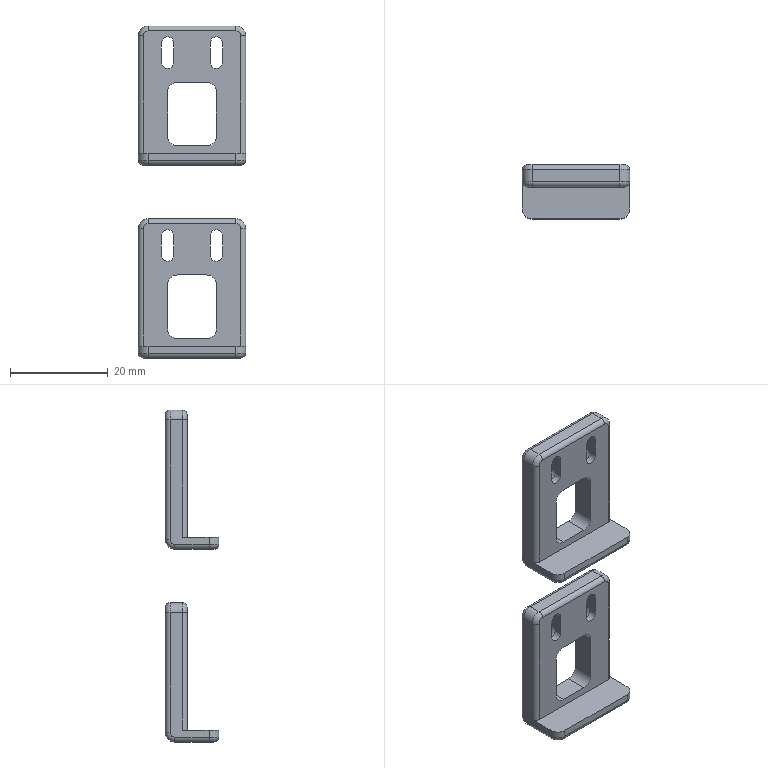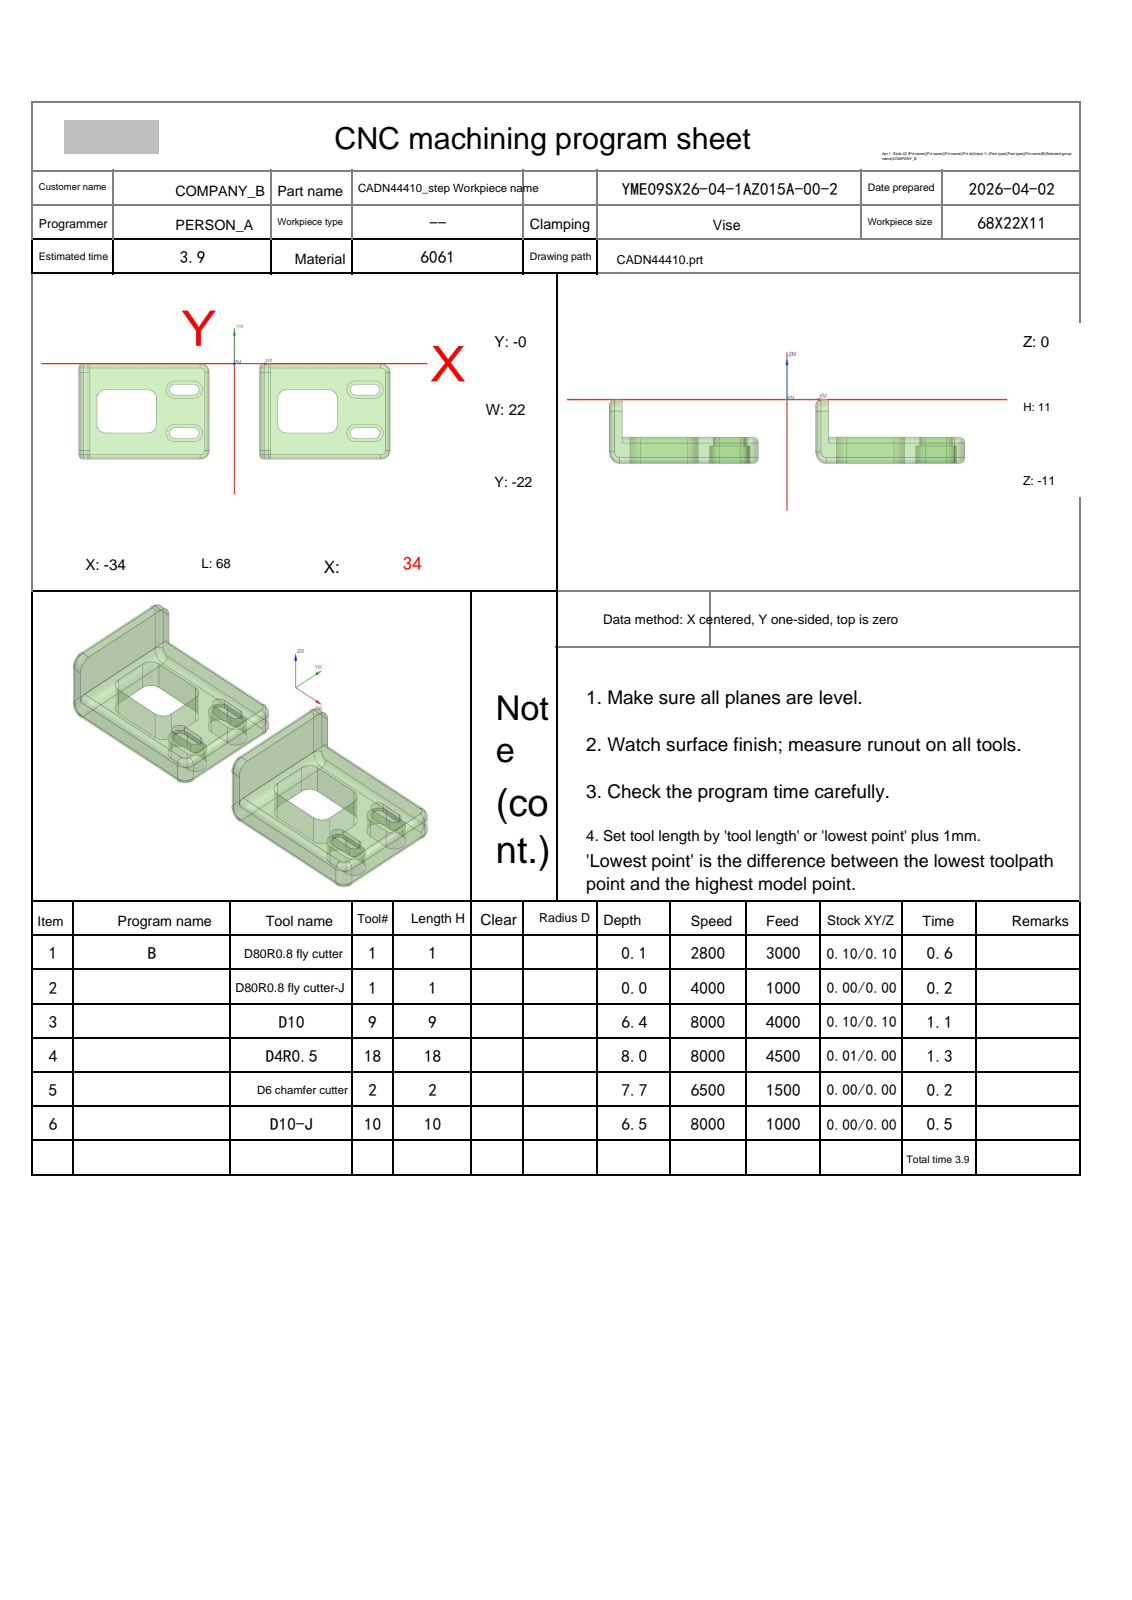NC program | NX | posted by the shop | part box 22 x 11 x 68 mm
Lines 1 to 1003 of 3177:
%
O0001
(Machine time: 5.00 MIN)
(===Total Tool:5===)
(T1=D80R0.8 fly cutter D=80.  R=0.8 H01 Z=0.    )
(T9=D10     D=10.  R=0.   D-  H09 Z=-6.4  )
(T18=D4R0.5 D=4.   R=0.5  D-  H18 Z=-8.   )
(T2=D6 chamfer cutter   D=6.   R=0.   D-  H02 Z=-7.7  )
(T10=D10-J  D=10.  R=0.   D10 H10 Z=-6.5  )
G80 G90 G17 G49 G40
G91 G28 Z0
M01
N1 T01 M06
(D80R0.8 fly cutter D=80. R=0.8 H=01 ce=0.10 di=0.10)
G00 G90 G54 X-86.097 Y-11. M03 S2800
G43 H01 Z20.
M08
Z5.513
G01 Z3.513 F3000.
X-74.097
X74.097
X86.097
Z5.513
G00 X-86.097
Z5.025
G01 Z3.025
X-74.097
X74.097
X86.097
Z5.025
G00 X-86.097
Z4.538
G01 Z2.538
X-74.097
X74.097
X86.097
Z4.538
G00 X-86.097
Z4.05
G01 Z2.05
X-74.097
X74.097
X86.097
Z4.05
G00 Z20.
X-86.097
Z3.563
G01 Z1.563
X-74.097
X74.097
X86.097
Z3.563
G00 Z20.
X-86.097
Z3.075
G01 Z1.075
X-74.097
X74.097
X86.097
Z3.075
G00 Z20.
X-86.097
Z2.588
G01 Z.588
X-74.097
X74.097
X86.097
Z2.588
G00 Z20.
X-86.097
Z2.1
G01 Z.1
X-74.097
X74.097
X86.097
Z2.1
G00 Z20.
G91 G28 Z0.0
M05
M09
G91 G28 Z0.0
M01
N2 T01 M06
(D80R0.8 fly cutter-J D=80. R=0.8 H=01 ce=0.00 di=0.00)
G00 G90 G54 X-85.999 Y-11. M03 S4000
G43 H01 Z20.
M08
Z2.
G01 Z0.0 F1000.
X-73.999
X73.999
X85.999
Z2.
G00 Z20.
G91 G28 Z0.0
M05
M09
G91 G28 Z0.0
M01
N3 T09 M06
(D10  D=10. R=0. H=09 ce=0.10 di=0.10)
G00 G90 G54 X-13.025 Y7. M03 S8000
G43 H09 Z13.5
M08
Z.918
G01 Z-.582 F4000.
Y3.9
X-7.5
G02 X-7.1 Y3.886 I0.0 J-5.9
X-5.689 Y3.615 I-.4 J-5.886
G01 X2.725 Y3.792
G03 X.4 Y-1. I3.775 J-4.792
G01 Y-21.
G03 X2.725 Y-25.792 I6.1 J0.0
G01 X-5.689 Y-25.615
X-5.705 Y-25.62
G02 X-7.5 Y-25.9 I-1.795 J5.62
G01 X-26.45
Y3.9
X-16.06
G02 X-15.228 Y3.455 I0.0 J-1.
G01 X-10.822 Y-3.155
G03 X-9.99 Y-3.6 I.832 J.555
G01 X-8.098
G02 X-7.1 Y-4.598 I-.002 J-1.
G01 Y-17.402
G02 X-8.098 Y-18.4 I-1. J.002
G01 X-17.952
G02 X-18.95 Y-17.402 I.002 J1.
G01 Y-4.598
G02 X-17.952 Y-3.6 I1. J-.002
G01 X-15.844
G02 X-14.984 Y-4.089 I0.0 J-1.
G01 X-12.827 Y-7.714
G03 X-12.284 Y-8.151 I.859 J.512
G02 X-11.6 Y-9.098 I-.316 J-.949
G01 Y-12.902
G02 X-12.598 Y-13.9 I-1. J.002
G01 X-13.452
G02 X-14.45 Y-12.902 I.002 J1.
G01 Y-9.098
G02 X-13.452 Y-8.1 I1. J-.002
G01 X-13.025
X-12.598
X-12.525 Y-8.103
X-12.3 Y-5.111
Z.918
G00 X-13.025 Y7.
Z.336
G01 Z-1.164
Y3.9
X-7.5
G02 X-7.1 Y3.886 I0.0 J-5.9
X-5.689 Y3.615 I-.4 J-5.886
G01 X2.725 Y3.792
G03 X.4 Y-1. I3.775 J-4.792
G01 Y-21.
G03 X2.725 Y-25.792 I6.1 J0.0
G01 X-5.689 Y-25.615
X-5.705 Y-25.62
G02 X-7.5 Y-25.9 I-1.795 J5.62
G01 X-26.45
Y3.9
X-16.06
G02 X-15.228 Y3.455 I0.0 J-1.
G01 X-10.822 Y-3.155
G03 X-9.99 Y-3.6 I.832 J.555
G01 X-8.098
G02 X-7.1 Y-4.598 I-.002 J-1.
G01 Y-17.402
G02 X-8.098 Y-18.4 I-1. J.002
G01 X-17.952
G02 X-18.95 Y-17.402 I.002 J1.
G01 Y-4.598
G02 X-17.952 Y-3.6 I1. J-.002
G01 X-15.844
G02 X-14.984 Y-4.089 I0.0 J-1.
G01 X-12.827 Y-7.714
G03 X-12.284 Y-8.151 I.859 J.512
G02 X-11.6 Y-9.098 I-.316 J-.949
G01 Y-12.902
G02 X-12.598 Y-13.9 I-1. J.002
G01 X-13.452
G02 X-14.45 Y-12.902 I.002 J1.
G01 Y-9.098
G02 X-13.452 Y-8.1 I1. J-.002
G01 X-13.025
X-12.598
X-12.525 Y-8.103
X-12.3 Y-5.111
Z.336
G00 X-13.025 Y7.
Z-.245
G01 Z-1.745
Y3.9
X-7.5
G02 X-7.1 Y3.886 I0.0 J-5.9
X-5.689 Y3.615 I-.4 J-5.886
G01 X2.725 Y3.792
G03 X.4 Y-1. I3.775 J-4.792
G01 Y-21.
G03 X2.725 Y-25.792 I6.1 J0.0
G01 X-5.689 Y-25.615
X-5.705 Y-25.62
G02 X-7.5 Y-25.9 I-1.795 J5.62
G01 X-26.45
Y3.9
X-16.06
G02 X-15.228 Y3.455 I0.0 J-1.
G01 X-10.822 Y-3.155
G03 X-9.99 Y-3.6 I.832 J.555
G01 X-8.098
G02 X-7.1 Y-4.598 I-.002 J-1.
G01 Y-17.402
G02 X-8.098 Y-18.4 I-1. J.002
G01 X-17.952
G02 X-18.95 Y-17.402 I.002 J1.
G01 Y-4.598
G02 X-17.952 Y-3.6 I1. J-.002
G01 X-15.844
G02 X-14.984 Y-4.089 I0.0 J-1.
G01 X-12.827 Y-7.714
G03 X-12.284 Y-8.151 I.859 J.512
G02 X-11.6 Y-9.098 I-.316 J-.949
G01 Y-12.902
G02 X-12.598 Y-13.9 I-1. J.002
G01 X-13.452
G02 X-14.45 Y-12.902 I.002 J1.
G01 Y-9.098
G02 X-13.452 Y-8.1 I1. J-.002
G01 X-13.025
X-12.598
X-12.525 Y-8.103
X-12.3 Y-5.111
Z-.245
G00 X-13.025 Y7.
Z-.827
G01 Z-2.327
Y3.9
X-7.5
G02 X-7.1 Y3.886 I0.0 J-5.9
X-5.689 Y3.615 I-.4 J-5.886
G01 X2.725 Y3.792
G03 X.4 Y-1. I3.775 J-4.792
G01 Y-21.
G03 X2.725 Y-25.792 I6.1 J0.0
G01 X-5.689 Y-25.615
X-5.705 Y-25.62
G02 X-7.5 Y-25.9 I-1.795 J5.62
G01 X-26.45
Y3.9
X-16.06
G02 X-15.228 Y3.455 I0.0 J-1.
G01 X-10.822 Y-3.155
G03 X-9.99 Y-3.6 I.832 J.555
G01 X-8.098
G02 X-7.1 Y-4.598 I-.002 J-1.
G01 Y-17.402
G02 X-8.098 Y-18.4 I-1. J.002
G01 X-17.952
G02 X-18.95 Y-17.402 I.002 J1.
G01 Y-4.598
G02 X-17.952 Y-3.6 I1. J-.002
G01 X-15.844
G02 X-14.984 Y-4.089 I0.0 J-1.
G01 X-12.827 Y-7.714
G03 X-12.284 Y-8.151 I.859 J.512
G02 X-11.6 Y-9.098 I-.316 J-.949
G01 Y-12.902
G02 X-12.598 Y-13.9 I-1. J.002
G01 X-13.452
G02 X-14.45 Y-12.902 I.002 J1.
G01 Y-9.098
G02 X-13.452 Y-8.1 I1. J-.002
G01 X-13.025
X-12.598
X-12.525 Y-8.103
X-12.3 Y-5.111
Z-.827
G00 X-13.025 Y7.
Z-1.409
G01 Z-2.909
Y3.9
X-7.5
G02 X-7.1 Y3.886 I0.0 J-5.9
X-5.689 Y3.615 I-.4 J-5.886
G01 X2.725 Y3.792
G03 X.4 Y-1. I3.775 J-4.792
G01 Y-21.
G03 X2.725 Y-25.792 I6.1 J0.0
G01 X-5.689 Y-25.615
X-5.705 Y-25.62
G02 X-7.5 Y-25.9 I-1.795 J5.62
G01 X-26.45
Y3.9
X-16.06
G02 X-15.228 Y3.455 I0.0 J-1.
G01 X-10.822 Y-3.155
G03 X-9.99 Y-3.6 I.832 J.555
G01 X-8.098
G02 X-7.1 Y-4.598 I-.002 J-1.
G01 Y-17.402
G02 X-8.098 Y-18.4 I-1. J.002
G01 X-17.952
G02 X-18.95 Y-17.402 I.002 J1.
G01 Y-4.598
G02 X-17.952 Y-3.6 I1. J-.002
G01 X-15.844
G02 X-14.984 Y-4.089 I0.0 J-1.
G01 X-12.827 Y-7.714
G03 X-12.284 Y-8.151 I.859 J.512
G02 X-11.6 Y-9.098 I-.316 J-.949
G01 Y-12.902
G02 X-12.598 Y-13.9 I-1. J.002
G01 X-13.452
G02 X-14.45 Y-12.902 I.002 J1.
G01 Y-9.098
G02 X-13.452 Y-8.1 I1. J-.002
G01 X-13.025
X-12.598
X-12.525 Y-8.103
X-12.3 Y-5.111
Z-1.409
G00 X-13.025 Y7.
Z-1.991
G01 Z-3.491
Y3.9
X-7.5
G02 X-7.1 Y3.886 I0.0 J-5.9
X-5.689 Y3.615 I-.4 J-5.886
G01 X2.725 Y3.792
G03 X.4 Y-1. I3.775 J-4.792
G01 Y-21.
G03 X2.725 Y-25.792 I6.1 J0.0
G01 X-5.689 Y-25.615
X-5.705 Y-25.62
G02 X-7.5 Y-25.9 I-1.795 J5.62
G01 X-26.45
Y3.9
X-16.06
G02 X-15.228 Y3.455 I0.0 J-1.
G01 X-10.822 Y-3.155
G03 X-9.99 Y-3.6 I.832 J.555
G01 X-8.098
G02 X-7.1 Y-4.598 I-.002 J-1.
G01 Y-17.402
G02 X-8.098 Y-18.4 I-1. J.002
G01 X-17.952
G02 X-18.95 Y-17.402 I.002 J1.
G01 Y-4.598
G02 X-17.952 Y-3.6 I1. J-.002
G01 X-15.844
G02 X-14.984 Y-4.089 I0.0 J-1.
G01 X-12.827 Y-7.714
G03 X-12.284 Y-8.151 I.859 J.512
G02 X-11.6 Y-9.098 I-.316 J-.949
G01 Y-12.902
G02 X-12.598 Y-13.9 I-1. J.002
G01 X-13.452
G02 X-14.45 Y-12.902 I.002 J1.
G01 Y-9.098
G02 X-13.452 Y-8.1 I1. J-.002
G01 X-13.025
X-12.598
X-12.525 Y-8.103
X-12.3 Y-5.111
Z-1.991
G00 X-13.025 Y7.
Z-2.573
G01 Z-4.073
Y3.9
X-7.5
G02 X-7.1 Y3.886 I0.0 J-5.9
X-5.689 Y3.615 I-.4 J-5.886
G01 X2.725 Y3.792
G03 X.4 Y-1. I3.775 J-4.792
G01 Y-21.
G03 X2.725 Y-25.792 I6.1 J0.0
G01 X-5.689 Y-25.615
X-5.705 Y-25.62
G02 X-7.5 Y-25.9 I-1.795 J5.62
G01 X-26.45
Y3.9
X-16.06
G02 X-15.228 Y3.455 I0.0 J-1.
G01 X-10.822 Y-3.155
G03 X-9.99 Y-3.6 I.832 J.555
G01 X-8.098
G02 X-7.1 Y-4.598 I-.002 J-1.
G01 Y-17.402
G02 X-8.098 Y-18.4 I-1. J.002
G01 X-17.952
G02 X-18.95 Y-17.402 I.002 J1.
G01 Y-4.598
G02 X-17.952 Y-3.6 I1. J-.002
G01 X-15.844
G02 X-14.984 Y-4.089 I0.0 J-1.
G01 X-12.827 Y-7.714
G03 X-12.284 Y-8.151 I.859 J.512
G02 X-11.6 Y-9.098 I-.316 J-.949
G01 Y-12.902
G02 X-12.598 Y-13.9 I-1. J.002
G01 X-13.452
G02 X-14.45 Y-12.902 I.002 J1.
G01 Y-9.098
G02 X-13.452 Y-8.1 I1. J-.002
G01 X-13.025
X-12.598
X-12.525 Y-8.103
X-12.3 Y-5.111
Z-2.573
G00 X-13.025 Y7.
Z-3.155
G01 Z-4.655
Y3.9
X-7.5
G02 X-7.1 Y3.886 I0.0 J-5.9
X-5.689 Y3.615 I-.4 J-5.886
G01 X2.725 Y3.792
G03 X.4 Y-1. I3.775 J-4.792
G01 Y-21.
G03 X2.725 Y-25.792 I6.1 J0.0
G01 X-5.689 Y-25.615
X-5.705 Y-25.62
G02 X-7.5 Y-25.9 I-1.795 J5.62
G01 X-26.45
Y3.9
X-16.06
G02 X-15.228 Y3.455 I0.0 J-1.
G01 X-10.822 Y-3.155
G03 X-9.99 Y-3.6 I.832 J.555
G01 X-8.098
G02 X-7.1 Y-4.598 I-.002 J-1.
G01 Y-17.402
G02 X-8.098 Y-18.4 I-1. J.002
G01 X-17.952
G02 X-18.95 Y-17.402 I.002 J1.
G01 Y-4.598
G02 X-17.952 Y-3.6 I1. J-.002
G01 X-15.844
G02 X-14.984 Y-4.089 I0.0 J-1.
G01 X-12.827 Y-7.714
G03 X-12.284 Y-8.151 I.859 J.512
G02 X-11.6 Y-9.098 I-.316 J-.949
G01 Y-12.902
G02 X-12.598 Y-13.9 I-1. J.002
G01 X-13.452
G02 X-14.45 Y-12.902 I.002 J1.
G01 Y-9.098
G02 X-13.452 Y-8.1 I1. J-.002
G01 X-13.025
X-12.598
X-12.525 Y-8.103
X-12.3 Y-5.111
Z-3.155
G00 X-13.025 Y7.
Z-3.736
G01 Z-5.236
Y3.9
X-7.5
G02 X-7.1 Y3.886 I0.0 J-5.9
X-5.689 Y3.615 I-.4 J-5.886
G01 X2.725 Y3.792
G03 X.4 Y-1. I3.775 J-4.792
G01 Y-21.
G03 X2.725 Y-25.792 I6.1 J0.0
G01 X-5.689 Y-25.615
X-5.705 Y-25.62
G02 X-7.5 Y-25.9 I-1.795 J5.62
G01 X-26.45
Y3.9
X-16.06
G02 X-15.228 Y3.455 I0.0 J-1.
G01 X-10.822 Y-3.155
G03 X-9.99 Y-3.6 I.832 J.555
G01 X-8.098
G02 X-7.1 Y-4.598 I-.002 J-1.
G01 Y-17.402
G02 X-8.098 Y-18.4 I-1. J.002
G01 X-17.952
G02 X-18.95 Y-17.402 I.002 J1.
G01 Y-4.598
G02 X-17.952 Y-3.6 I1. J-.002
G01 X-15.844
G02 X-14.984 Y-4.089 I0.0 J-1.
G01 X-12.827 Y-7.714
G03 X-12.284 Y-8.151 I.859 J.512
G02 X-11.6 Y-9.098 I-.316 J-.949
G01 Y-12.902
G02 X-12.598 Y-13.9 I-1. J.002
G01 X-13.452
G02 X-14.45 Y-12.902 I.002 J1.
G01 Y-9.098
G02 X-13.452 Y-8.1 I1. J-.002
G01 X-13.025
X-12.598
X-12.525 Y-8.103
X-12.3 Y-5.111
Z-3.736
G00 X-13.025 Y7.
Z-4.318
G01 Z-5.818
Y3.9
X-7.5
G02 X-7.1 Y3.886 I0.0 J-5.9
X-5.689 Y3.615 I-.4 J-5.886
G01 X2.725 Y3.792
G03 X.4 Y-1. I3.775 J-4.792
G01 Y-21.
G03 X2.725 Y-25.792 I6.1 J0.0
G01 X-5.689 Y-25.615
X-5.705 Y-25.62
G02 X-7.5 Y-25.9 I-1.795 J5.62
G01 X-26.45
Y3.9
X-16.06
G02 X-15.228 Y3.455 I0.0 J-1.
G01 X-10.822 Y-3.155
G03 X-9.99 Y-3.6 I.832 J.555
G01 X-8.098
G02 X-7.1 Y-4.598 I-.002 J-1.
G01 Y-17.402
G02 X-8.098 Y-18.4 I-1. J.002
G01 X-17.952
G02 X-18.95 Y-17.402 I.002 J1.
G01 Y-4.598
G02 X-17.952 Y-3.6 I1. J-.002
G01 X-15.844
G02 X-14.984 Y-4.089 I0.0 J-1.
G01 X-12.827 Y-7.714
G03 X-12.284 Y-8.151 I.859 J.512
G02 X-11.6 Y-9.098 I-.316 J-.949
G01 Y-12.902
G02 X-12.598 Y-13.9 I-1. J.002
G01 X-13.452
G02 X-14.45 Y-12.902 I.002 J1.
G01 Y-9.098
G02 X-13.452 Y-8.1 I1. J-.002
G01 X-13.025
X-12.598
X-12.525 Y-8.103
X-12.3 Y-5.111
Z-4.318
G00 X-13.025 Y7.
Z-4.9
G01 Z-6.4
Y3.9
X-7.5
G02 X-7.1 Y3.886 I0.0 J-5.9
X-5.689 Y3.615 I-.4 J-5.886
G01 X2.725 Y3.792
G03 X.4 Y-1. I3.775 J-4.792
G01 Y-21.
G03 X2.725 Y-25.792 I6.1 J0.0
G01 X-5.689 Y-25.615
X-5.705 Y-25.62
G02 X-7.5 Y-25.9 I-1.795 J5.62
G01 X-26.45
Y3.9
X-16.06
G02 X-15.228 Y3.455 I0.0 J-1.
G01 X-10.822 Y-3.155
G03 X-9.99 Y-3.6 I.832 J.555
G01 X-8.098
G02 X-7.1 Y-4.598 I-.002 J-1.
G01 Y-17.402
G02 X-8.098 Y-18.4 I-1. J.002
G01 X-17.952
G02 X-18.95 Y-17.402 I.002 J1.
G01 Y-4.598
G02 X-17.952 Y-3.6 I1. J-.002
G01 X-15.844
G02 X-14.984 Y-4.089 I0.0 J-1.
G01 X-12.827 Y-7.714
G03 X-12.284 Y-8.151 I.859 J.512
G02 X-11.6 Y-9.098 I-.316 J-.949
G01 Y-12.902
G02 X-12.598 Y-13.9 I-1. J.002
G01 X-13.452
G02 X-14.45 Y-12.902 I.002 J1.
G01 Y-9.098
G02 X-13.452 Y-8.1 I1. J-.002
G01 X-13.025
X-12.598
X-12.525 Y-8.103
X-12.3 Y-5.111
Z-4.9
G00 Z13.5
X41. Y-11.
Z.918
G01 Z-.582
X37.9
Y-20.
G02 X32. Y-25.9 I-5.9 J0.0
G01 X13.05
Y3.9
X32.
G02 X37.9 Y-2. I0.0 J-5.9
G01 Y-7.965
G02 X37.455 Y-8.797 I-1. J0.0
G01 X30.845 Y-13.203
G03 X30.4 Y-14.035 I.555 J-.832
G01 Y-17.402
G02 X29.402 Y-18.4 I-1. J.002
G01 X21.548
G02 X20.55 Y-17.402 I.002 J1.
G01 Y-4.598
G02 X21.548 Y-3.6 I1. J-.002
G01 X29.402
G02 X30.4 Y-4.598 I-.002 J-1.
G01 Y-8.336
G02 X30.107 Y-9.043 I-1. J0.0
G01 X26.182 Y-12.968
G03 X25.897 Y-13.55 I.707 J-.707
G02 X25.502 Y-13.9 I-.397 J.05
G01 X25.448
G02 X25.05 Y-13.502 I.002 J.4
G01 Y-8.498
G02 X25.448 Y-8.1 I.4 J-.002
G01 X25.502
G02 X25.9 Y-8.498 I-.002 J-.4
G01 Y-11.
Y-11.5
X28.9
Z.918
G00 X41. Y-11.
Z.336
G01 Z-1.164
X37.9
Y-20.
G02 X32. Y-25.9 I-5.9 J0.0
G01 X13.05
Y3.9
X32.
G02 X37.9 Y-2. I0.0 J-5.9
G01 Y-7.965
G02 X37.455 Y-8.797 I-1. J0.0
G01 X30.845 Y-13.203
G03 X30.4 Y-14.035 I.555 J-.832
G01 Y-17.402
G02 X29.402 Y-18.4 I-1. J.002
G01 X21.548
G02 X20.55 Y-17.402 I.002 J1.
G01 Y-4.598
G02 X21.548 Y-3.6 I1. J-.002
G01 X29.402
G02 X30.4 Y-4.598 I-.002 J-1.
G01 Y-8.336
G02 X30.107 Y-9.043 I-1. J0.0
G01 X26.182 Y-12.968
G03 X25.897 Y-13.55 I.707 J-.707
G02 X25.502 Y-13.9 I-.397 J.05
G01 X25.448
G02 X25.05 Y-13.502 I.002 J.4
G01 Y-8.498
G02 X25.448 Y-8.1 I.4 J-.002
G01 X25.502
G02 X25.9 Y-8.498 I-.002 J-.4
G01 Y-11.
Y-11.5
X28.9
Z.336
G00 X41. Y-11.
Z-.245
G01 Z-1.745
X37.9
Y-20.
G02 X32. Y-25.9 I-5.9 J0.0
G01 X13.05
Y3.9
X32.
G02 X37.9 Y-2. I0.0 J-5.9
G01 Y-7.965
G02 X37.455 Y-8.797 I-1. J0.0
G01 X30.845 Y-13.203
G03 X30.4 Y-14.035 I.555 J-.832
G01 Y-17.402
G02 X29.402 Y-18.4 I-1. J.002
G01 X21.548
G02 X20.55 Y-17.402 I.002 J1.
G01 Y-4.598
G02 X21.548 Y-3.6 I1. J-.002
G01 X29.402
G02 X30.4 Y-4.598 I-.002 J-1.
G01 Y-8.336
G02 X30.107 Y-9.043 I-1. J0.0
G01 X26.182 Y-12.968
G03 X25.897 Y-13.55 I.707 J-.707
G02 X25.502 Y-13.9 I-.397 J.05
G01 X25.448
G02 X25.05 Y-13.502 I.002 J.4
G01 Y-8.498
G02 X25.448 Y-8.1 I.4 J-.002
G01 X25.502
G02 X25.9 Y-8.498 I-.002 J-.4
G01 Y-11.
Y-11.5
X28.9
Z-.245
G00 X41. Y-11.
Z-.827
G01 Z-2.327
X37.9
Y-20.
G02 X32. Y-25.9 I-5.9 J0.0
G01 X13.05
Y3.9
X32.
G02 X37.9 Y-2. I0.0 J-5.9
G01 Y-7.965
G02 X37.455 Y-8.797 I-1. J0.0
G01 X30.845 Y-13.203
G03 X30.4 Y-14.035 I.555 J-.832
G01 Y-17.402
G02 X29.402 Y-18.4 I-1. J.002
G01 X21.548
G02 X20.55 Y-17.402 I.002 J1.
G01 Y-4.598
G02 X21.548 Y-3.6 I1. J-.002
G01 X29.402
G02 X30.4 Y-4.598 I-.002 J-1.
G01 Y-8.336
G02 X30.107 Y-9.043 I-1. J0.0
G01 X26.182 Y-12.968
G03 X25.897 Y-13.55 I.707 J-.707
G02 X25.502 Y-13.9 I-.397 J.05
G01 X25.448
G02 X25.05 Y-13.502 I.002 J.4
G01 Y-8.498
G02 X25.448 Y-8.1 I.4 J-.002
G01 X25.502
G02 X25.9 Y-8.498 I-.002 J-.4
G01 Y-11.
Y-11.5
X28.9
Z-.827
G00 X41. Y-11.
Z-1.409
G01 Z-2.909
X37.9
Y-20.
G02 X32. Y-25.9 I-5.9 J0.0
G01 X13.05
Y3.9
X32.
G02 X37.9 Y-2. I0.0 J-5.9
G01 Y-7.965
G02 X37.455 Y-8.797 I-1. J0.0
G01 X30.845 Y-13.203
G03 X30.4 Y-14.035 I.555 J-.832
G01 Y-17.402
G02 X29.402 Y-18.4 I-1. J.002
G01 X21.548
G02 X20.55 Y-17.402 I.002 J1.
G01 Y-4.598
G02 X21.548 Y-3.6 I1. J-.002
G01 X29.402
G02 X30.4 Y-4.598 I-.002 J-1.
G01 Y-8.336
G02 X30.107 Y-9.043 I-1. J0.0
G01 X26.182 Y-12.968
G03 X25.897 Y-13.55 I.707 J-.707
G02 X25.502 Y-13.9 I-.397 J.05
G01 X25.448
G02 X25.05 Y-13.502 I.002 J.4
G01 Y-8.498
G02 X25.448 Y-8.1 I.4 J-.002
G01 X25.502
G02 X25.9 Y-8.498 I-.002 J-.4
G01 Y-11.
Y-11.5
X28.9
Z-1.409
G00 X41. Y-11.
Z-1.991
G01 Z-3.491
X37.9
Y-20.
G02 X32. Y-25.9 I-5.9 J0.0
G01 X13.05
Y3.9
X32.
G02 X37.9 Y-2. I0.0 J-5.9
G01 Y-7.965
G02 X37.455 Y-8.797 I-1. J0.0
G01 X30.845 Y-13.203
G03 X30.4 Y-14.035 I.555 J-.832
G01 Y-17.402
G02 X29.402 Y-18.4 I-1. J.002
G01 X21.548
G02 X20.55 Y-17.402 I.002 J1.
G01 Y-4.598
G02 X21.548 Y-3.6 I1. J-.002
G01 X29.402
G02 X30.4 Y-4.598 I-.002 J-1.
G01 Y-8.336
G02 X30.107 Y-9.043 I-1. J0.0
G01 X26.182 Y-12.968
G03 X25.897 Y-13.55 I.707 J-.707
G02 X25.502 Y-13.9 I-.397 J.05
G01 X25.448
G02 X25.05 Y-13.502 I.002 J.4
G01 Y-8.498
G02 X25.448 Y-8.1 I.4 J-.002
G01 X25.502
G02 X25.9 Y-8.498 I-.002 J-.4
G01 Y-11.
Y-11.5
X28.9
Z-1.991
G00 X41. Y-11.
Z-2.573
G01 Z-4.073
X37.9
Y-20.
G02 X32. Y-25.9 I-5.9 J0.0
G01 X13.05
Y3.9
X32.
G02 X37.9 Y-2. I0.0 J-5.9
G01 Y-7.965
G02 X37.455 Y-8.797 I-1. J0.0
G01 X30.845 Y-13.203
G03 X30.4 Y-14.035 I.555 J-.832
G01 Y-17.402
G02 X29.402 Y-18.4 I-1. J.002
G01 X21.548
G02 X20.55 Y-17.402 I.002 J1.
G01 Y-4.598
G02 X21.548 Y-3.6 I1. J-.002
G01 X29.402
G02 X30.4 Y-4.598 I-.002 J-1.
G01 Y-8.336
G02 X30.107 Y-9.043 I-1. J0.0
G01 X26.182 Y-12.968
G03 X25.897 Y-13.55 I.707 J-.707
G02 X25.502 Y-13.9 I-.397 J.05
G01 X25.448
G02 X25.05 Y-13.502 I.002 J.4
G01 Y-8.498
G02 X25.448 Y-8.1 I.4 J-.002
G01 X25.502
G02 X25.9 Y-8.498 I-.002 J-.4
G01 Y-11.
Y-11.5
X28.9
Z-2.573
G00 X41. Y-11.
Z-3.155
G01 Z-4.655
X37.9
Y-20.
G02 X32. Y-25.9 I-5.9 J0.0
G01 X13.05
Y3.9
X32.
G02 X37.9 Y-2. I0.0 J-5.9
G01 Y-7.965
G02 X37.455 Y-8.797 I-1. J0.0
G01 X30.845 Y-13.203
G03 X30.4 Y-14.035 I.555 J-.832
G01 Y-17.402
G02 X29.402 Y-18.4 I-1. J.002
G01 X21.548
G02 X20.55 Y-17.402 I.002 J1.
G01 Y-4.598
G02 X21.548 Y-3.6 I1. J-.002
G01 X29.402
G02 X30.4 Y-4.598 I-.002 J-1.
G01 Y-8.336
G02 X30.107 Y-9.043 I-1. J0.0
G01 X26.182 Y-12.968
G03 X25.897 Y-13.55 I.707 J-.707
G02 X25.502 Y-13.9 I-.397 J.05
G01 X25.448
G02 X25.05 Y-13.502 I.002 J.4
G01 Y-8.498
G02 X25.448 Y-8.1 I.4 J-.002
G01 X25.502
G02 X25.9 Y-8.498 I-.002 J-.4
G01 Y-11.
Y-11.5
X28.9
Z-3.155
G00 X41. Y-11.
Z-3.736
G01 Z-5.236
X37.9
Y-20.
G02 X32. Y-25.9 I-5.9 J0.0
G01 X13.05
Y3.9
X32.
G02 X37.9 Y-2. I0.0 J-5.9
G01 Y-7.965
G02 X37.455 Y-8.797 I-1. J0.0
G01 X30.845 Y-13.203
G03 X30.4 Y-14.035 I.555 J-.832
G01 Y-17.402
G02 X29.402 Y-18.4 I-1. J.002
G01 X21.548
G02 X20.55 Y-17.402 I.002 J1.
G01 Y-4.598
G02 X21.548 Y-3.6 I1. J-.002
G01 X29.402
G02 X30.4 Y-4.598 I-.002 J-1.
G01 Y-8.336
G02 X30.107 Y-9.043 I-1. J0.0
G01 X26.182 Y-12.968
G03 X25.897 Y-13.55 I.707 J-.707
G02 X25.502 Y-13.9 I-.397 J.05
G01 X25.448
G02 X25.05 Y-13.502 I.002 J.4
G01 Y-8.498
G02 X25.448 Y-8.1 I.4 J-.002
G01 X25.502
G02 X25.9 Y-8.498 I-.002 J-.4
G01 Y-11.
Y-11.5
X28.9
Z-3.736
G00 X41. Y-11.
Z-4.318
G01 Z-5.818
X37.9
Y-20.
G02 X32. Y-25.9 I-5.9 J0.0
G01 X13.05
Y3.9
X32.
G02 X37.9 Y-2. I0.0 J-5.9
G01 Y-7.965
G02 X37.455 Y-8.797 I-1. J0.0
G01 X30.845 Y-13.203
G03 X30.4 Y-14.035 I.555 J-.832
G01 Y-17.402
G02 X29.402 Y-18.4 I-1. J.002
G01 X21.548
G02 X20.55 Y-17.402 I.002 J1.
G01 Y-4.598
G02 X21.548 Y-3.6 I1. J-.002
G01 X29.402
G02 X30.4 Y-4.598 I-.002 J-1.
G01 Y-8.336
G02 X30.107 Y-9.043 I-1. J0.0
G01 X26.182 Y-12.968
G03 X25.897 Y-13.55 I.707 J-.707
G02 X25.502 Y-13.9 I-.397 J.05
G01 X25.448
G02 X25.05 Y-13.502 I.002 J.4
G01 Y-8.498
G02 X25.448 Y-8.1 I.4 J-.002
G01 X25.502
G02 X25.9 Y-8.498 I-.002 J-.4
G01 Y-11.
Y-11.5
X28.9
Z-4.318
G00 X41. Y-11.
Z-4.9
G01 Z-6.4
X37.9
Y-20.
G02 X32. Y-25.9 I-5.9 J0.0
G01 X13.05
Y3.9
X32.
G02 X37.9 Y-2. I0.0 J-5.9
G01 Y-7.965
G02 X37.455 Y-8.797 I-1. J0.0
G01 X30.845 Y-13.203
G03 X30.4 Y-14.035 I.555 J-.832
G01 Y-17.402
G02 X29.402 Y-18.4 I-1. J.002
G01 X21.548
G02 X20.55 Y-17.402 I.002 J1.
G01 Y-4.598
G02 X21.548 Y-3.6 I1. J-.002
G01 X29.402
G02 X30.4 Y-4.598 I-.002 J-1.
G01 Y-8.336
G02 X30.107 Y-9.043 I-1. J0.0
G01 X26.182 Y-12.968
G03 X25.897 Y-13.55 I.707 J-.707
G02 X25.502 Y-13.9 I-.397 J.05
G01 X25.448
G02 X25.05 Y-13.502 I.002 J.4
G01 Y-8.498
G02 X25.448 Y-8.1 I.4 J-.002
G01 X25.502
G02 X25.9 Y-8.498 I-.002 J-.4
G01 Y-11.
Y-11.5
X28.9
Z-4.9
G00 Z13.5
G91 G28 Z0.0
M05
M09
G91 G28 Z0.0
M01